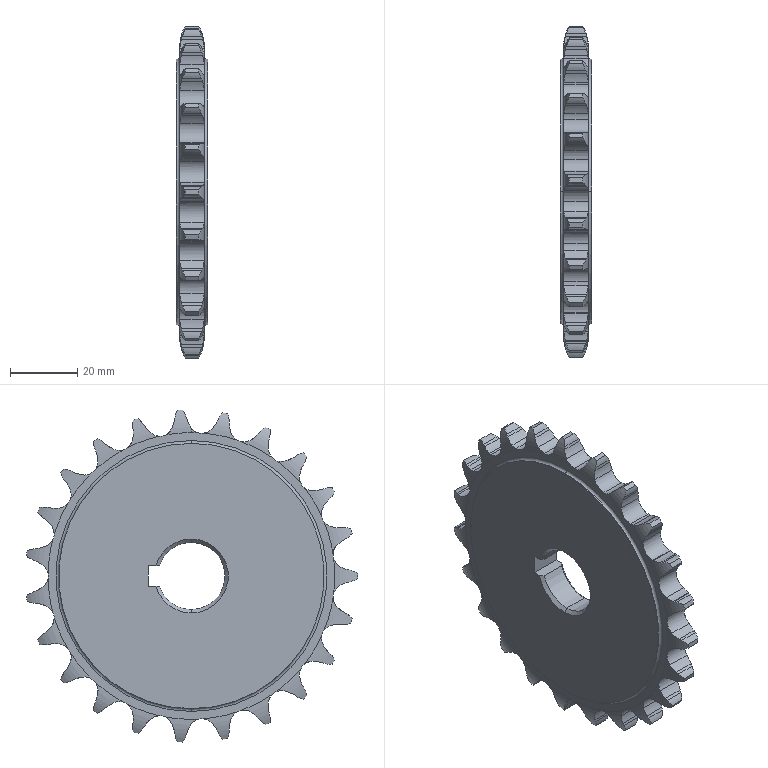Part | SolidWorks | features Chamfer 3, Cut 2, Revolution 2, CirPattern 1 | 1 solid | 268 faces | box 9.37 x 98.633 x 98.858 mm | volume 53510 mm3 | cylinder 157 | plane 53 | torus 52 | cone 6 | commonest cylinder face diameters 11.437 x49 20.732 x48 8.06 x30 99 x23 79 x4 20 x3